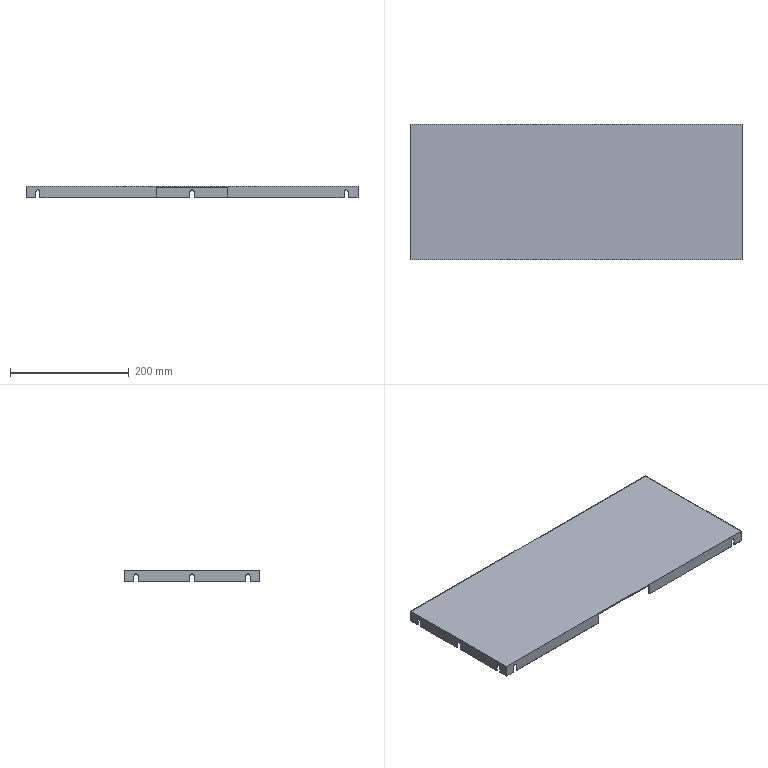Part | STEP file | PN_0020 | 1 solid | 63 faces | box 558 x 228 x 20 mm | volume 153874 mm3 | plane 47 | cylinder 16 | commonest cylinder face diameters 7 x16